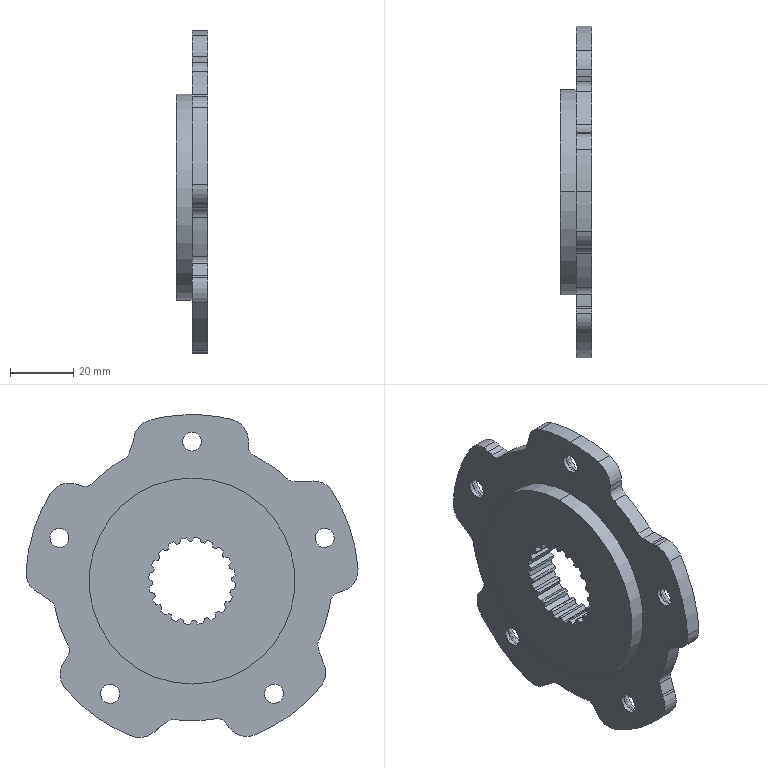Part | STEP file | Completa.sldasm-Part-21_Valor predeterminado | 1 solid | 173 faces | box 10 x 104.793 x 101.882 mm | volume 47802 mm3 | cylinder 80 | plane 73 | cone 10 | torus 10 | commonest cylinder face diameters 25 x20 6.496 x15 14 x12 6 x10 11.34 x10 105 x6